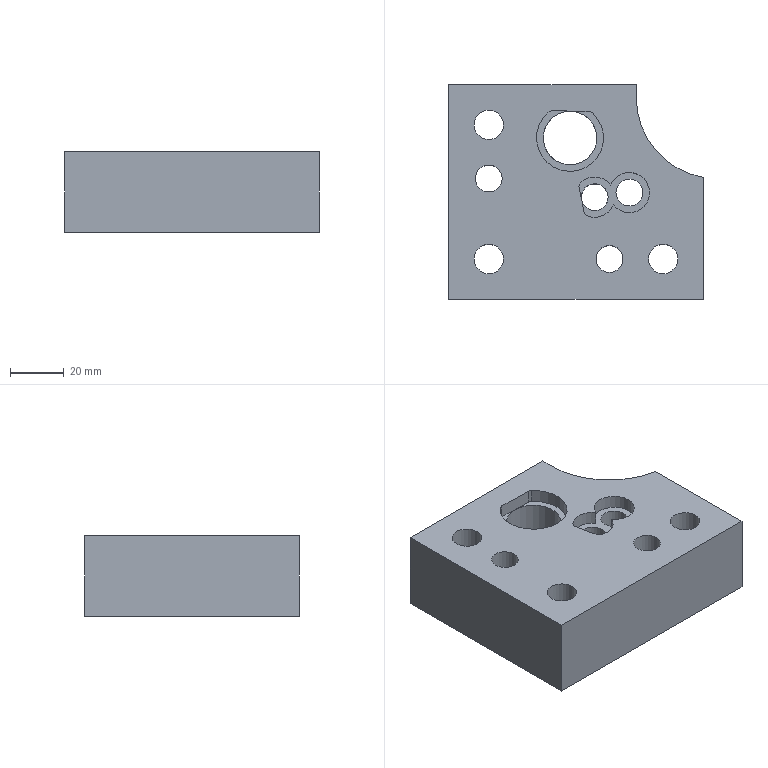Part | NX | features solid 2 | 1 solid | 34 faces | box 95 x 80 x 30 mm | volume 174573 mm3 | cylinder 20 | plane 14 | commonest cylinder face diameters 4 x4 10 x4 11 x3 15 x3 17 x3 20 x1
STEP:
#1=CARTESIAN_POINT('',(-403.57,200.221,109.));
#2=VERTEX_POINT('',#1);
#3=CARTESIAN_POINT('',(-404.546,207.571,109.));
#4=VERTEX_POINT('',#3);
#5=CARTESIAN_POINT('',(-397.595,204.754,109.));
#6=DIRECTION('',(0.,0.,-1.));
#7=DIRECTION('',(-1.,0.,0.));
#8=AXIS2_PLACEMENT_3D('',#5,#6,#7);
#9=CIRCLE('',#8,7.5);
#10=EDGE_CURVE('',#2,#4,#9,.F.);
#11=ORIENTED_EDGE('',*,*,#10,.F.);
#12=CARTESIAN_POINT('',(-413.225,196.042,109.));
#13=VERTEX_POINT('',#12);
#14=CARTESIAN_POINT('',(-410.521,203.038,109.));
#15=DIRECTION('',(0.,0.,-1.));
#16=DIRECTION('',(-1.,0.,0.));
#17=AXIS2_PLACEMENT_3D('',#14,#15,#16);
#18=CIRCLE('',#17,7.5);
#19=EDGE_CURVE('',#13,#2,#18,.F.);
#20=ORIENTED_EDGE('',*,*,#19,.F.);
#21=CARTESIAN_POINT('',(-414.461,197.494,109.));
#22=VERTEX_POINT('',#21);
#23=CARTESIAN_POINT('',(-412.504,197.908,109.));
#24=DIRECTION('',(0.,0.,-1.));
#25=DIRECTION('',(-1.,0.,0.));
#26=AXIS2_PLACEMENT_3D('',#23,#24,#25);
#27=CIRCLE('',#26,2.);
#28=EDGE_CURVE('',#13,#22,#27,.T.);
#29=ORIENTED_EDGE('',*,*,#28,.T.);
#30=CARTESIAN_POINT('',(-416.366,206.515,109.));
#31=VERTEX_POINT('',#30);
#32=CARTESIAN_POINT('',(-422.167,233.981,109.));
#33=DIRECTION('',(-0.2067,0.9784,0.));
#34=VECTOR('',#33,1000.);
#35=LINE('',#32,#34);
#36=EDGE_CURVE('',#22,#31,#35,.T.);
#37=ORIENTED_EDGE('',*,*,#36,.T.);
#38=CARTESIAN_POINT('',(-415.823,208.343,109.));
#39=VERTEX_POINT('',#38);
#40=CARTESIAN_POINT('',(-414.409,206.928,109.));
#41=DIRECTION('',(0.,0.,-1.));
#42=DIRECTION('',(-1.,0.,0.));
#43=AXIS2_PLACEMENT_3D('',#40,#41,#42);
#44=CIRCLE('',#43,2.);
#45=EDGE_CURVE('',#31,#39,#44,.T.);
#46=ORIENTED_EDGE('',*,*,#45,.T.);
#47=CARTESIAN_POINT('',(-410.521,203.038,109.));
#48=DIRECTION('',(0.,0.,-1.));
#49=DIRECTION('',(-1.,0.,0.));
#50=AXIS2_PLACEMENT_3D('',#47,#48,#49);
#51=CIRCLE('',#50,7.5);
#52=EDGE_CURVE('',#4,#39,#51,.F.);
#53=ORIENTED_EDGE('',*,*,#52,.F.);
#54=EDGE_LOOP('',(#11,#20,#29,#37,#46,#53));
#55=FACE_BOUND('',#54,.T.);
#56=CARTESIAN_POINT('',(-427.542,234.881,109.));
#57=VERTEX_POINT('',#56);
#58=CARTESIAN_POINT('',(-411.356,234.431,109.));
#59=VERTEX_POINT('',#58);
#60=CARTESIAN_POINT('',(-419.714,225.136,109.));
#61=DIRECTION('',(0.,0.,-1.));
#62=DIRECTION('',(-1.,0.,0.));
#63=AXIS2_PLACEMENT_3D('',#60,#61,#62);
#64=CIRCLE('',#63,12.5);
#65=EDGE_CURVE('',#57,#59,#64,.F.);
#66=ORIENTED_EDGE('',*,*,#65,.F.);
#67=CARTESIAN_POINT('',(-426.234,235.321,109.));
#68=VERTEX_POINT('',#67);
#69=CARTESIAN_POINT('',(-426.29,233.322,109.));
#70=DIRECTION('',(0.,0.,-1.));
#71=DIRECTION('',(-1.,0.,0.));
#72=AXIS2_PLACEMENT_3D('',#69,#70,#71);
#73=CIRCLE('',#72,2.);
#74=EDGE_CURVE('',#57,#68,#73,.T.);
#75=ORIENTED_EDGE('',*,*,#74,.T.);
#76=CARTESIAN_POINT('',(-412.638,234.943,109.));
#77=VERTEX_POINT('',#76);
#78=CARTESIAN_POINT('',(-370.312,233.766,109.));
#79=DIRECTION('',(0.9996,-0.0278,0.));
#80=VECTOR('',#79,1000.);
#81=LINE('',#78,#80);
#82=EDGE_CURVE('',#68,#77,#81,.T.);
#83=ORIENTED_EDGE('',*,*,#82,.T.);
#84=CARTESIAN_POINT('',(-412.693,232.944,109.));
#85=DIRECTION('',(0.,0.,-1.));
#86=DIRECTION('',(-1.,0.,0.));
#87=AXIS2_PLACEMENT_3D('',#84,#85,#86);
#88=CIRCLE('',#87,2.);
#89=EDGE_CURVE('',#77,#59,#88,.T.);
#90=ORIENTED_EDGE('',*,*,#89,.T.);
#91=EDGE_LOOP('',(#66,#75,#83,#90));
#92=FACE_BOUND('',#91,.T.);
#93=CARTESIAN_POINT('',(-455.5,180.,109.));
#94=VERTEX_POINT('',#93);
#95=CARTESIAN_POINT('',(-450.,180.,109.));
#96=DIRECTION('',(0.,0.,-1.));
#97=DIRECTION('',(-1.,0.,0.));
#98=AXIS2_PLACEMENT_3D('',#95,#96,#97);
#99=CIRCLE('',#98,5.5);
#100=EDGE_CURVE('',#94,#94,#99,.T.);
#101=ORIENTED_EDGE('',*,*,#100,.T.);
#102=EDGE_LOOP('',(#101));
#103=FACE_BOUND('',#102,.T.);
#104=CARTESIAN_POINT('',(-455.5,230.,109.));
#105=VERTEX_POINT('',#104);
#106=CARTESIAN_POINT('',(-450.,230.,109.));
#107=DIRECTION('',(0.,0.,-1.));
#108=DIRECTION('',(-1.,0.,0.));
#109=AXIS2_PLACEMENT_3D('',#106,#107,#108);
#110=CIRCLE('',#109,5.5);
#111=EDGE_CURVE('',#105,#105,#110,.T.);
#112=ORIENTED_EDGE('',*,*,#111,.T.);
#113=EDGE_LOOP('',(#112));
#114=FACE_BOUND('',#113,.T.);
#115=CARTESIAN_POINT('',(-390.5,180.,109.));
#116=VERTEX_POINT('',#115);
#117=CARTESIAN_POINT('',(-385.,180.,109.));
#118=DIRECTION('',(0.,0.,-1.));
#119=DIRECTION('',(-1.,0.,0.));
#120=AXIS2_PLACEMENT_3D('',#117,#118,#119);
#121=CIRCLE('',#120,5.5);
#122=EDGE_CURVE('',#116,#116,#121,.T.);
#123=ORIENTED_EDGE('',*,*,#122,.T.);
#124=EDGE_LOOP('',(#123));
#125=FACE_BOUND('',#124,.T.);
#126=CARTESIAN_POINT('',(-455.,210.,109.));
#127=VERTEX_POINT('',#126);
#128=CARTESIAN_POINT('',(-450.,210.,109.));
#129=DIRECTION('',(0.,0.,-1.));
#130=DIRECTION('',(-1.,0.,0.));
#131=AXIS2_PLACEMENT_3D('',#128,#129,#130);
#132=CIRCLE('',#131,5.);
#133=EDGE_CURVE('',#127,#127,#132,.T.);
#134=ORIENTED_EDGE('',*,*,#133,.T.);
#135=EDGE_LOOP('',(#134));
#136=FACE_BOUND('',#135,.T.);
#137=CARTESIAN_POINT('',(-410.,180.,109.));
#138=VERTEX_POINT('',#137);
#139=CARTESIAN_POINT('',(-405.,180.,109.));
#140=DIRECTION('',(0.,0.,-1.));
#141=DIRECTION('',(-1.,0.,0.));
#142=AXIS2_PLACEMENT_3D('',#139,#140,#141);
#143=CIRCLE('',#142,5.);
#144=EDGE_CURVE('',#138,#138,#143,.T.);
#145=ORIENTED_EDGE('',*,*,#144,.T.);
#146=EDGE_LOOP('',(#145));
#147=FACE_BOUND('',#146,.T.);
#148=CARTESIAN_POINT('',(-395.,245.,109.));
#149=VERTEX_POINT('',#148);
#150=CARTESIAN_POINT('',(-395.,240.,109.));
#151=VERTEX_POINT('',#150);
#152=CARTESIAN_POINT('',(-395.,245.,109.));
#153=DIRECTION('',(0.,-1.,0.));
#154=VECTOR('',#153,1000.);
#155=LINE('',#152,#154);
#156=EDGE_CURVE('',#149,#151,#155,.T.);
#157=ORIENTED_EDGE('',*,*,#156,.F.);
#158=CARTESIAN_POINT('',(-465.,245.,109.));
#159=VERTEX_POINT('',#158);
#160=CARTESIAN_POINT('',(-465.,245.,109.));
#161=DIRECTION('',(1.,0.,0.));
#162=VECTOR('',#161,1000.);
#163=LINE('',#160,#162);
#164=EDGE_CURVE('',#159,#149,#163,.T.);
#165=ORIENTED_EDGE('',*,*,#164,.F.);
#166=CARTESIAN_POINT('',(-465.,165.,109.));
#167=VERTEX_POINT('',#166);
#168=CARTESIAN_POINT('',(-465.,165.,109.));
#169=DIRECTION('',(0.,1.,0.));
#170=VECTOR('',#169,1000.);
#171=LINE('',#168,#170);
#172=EDGE_CURVE('',#167,#159,#171,.T.);
#173=ORIENTED_EDGE('',*,*,#172,.F.);
#174=CARTESIAN_POINT('',(-370.,165.,109.));
#175=VERTEX_POINT('',#174);
#176=CARTESIAN_POINT('',(-465.,165.,109.));
#177=DIRECTION('',(1.,0.,0.));
#178=VECTOR('',#177,1000.);
#179=LINE('',#176,#178);
#180=EDGE_CURVE('',#167,#175,#179,.T.);
#181=ORIENTED_EDGE('',*,*,#180,.T.);
#182=CARTESIAN_POINT('',(-370.,210.42,109.));
#183=VERTEX_POINT('',#182);
#184=CARTESIAN_POINT('',(-370.,165.,109.));
#185=DIRECTION('',(0.,1.,0.));
#186=VECTOR('',#185,1000.);
#187=LINE('',#184,#186);
#188=EDGE_CURVE('',#175,#183,#187,.T.);
#189=ORIENTED_EDGE('',*,*,#188,.T.);
#190=CARTESIAN_POINT('',(-365.,240.,109.));
#191=DIRECTION('',(0.,0.,-1.));
#192=DIRECTION('',(-1.,0.,0.));
#193=AXIS2_PLACEMENT_3D('',#190,#191,#192);
#194=CIRCLE('',#193,30.);
#195=EDGE_CURVE('',#183,#151,#194,.T.);
#196=ORIENTED_EDGE('',*,*,#195,.T.);
#197=EDGE_LOOP('',(#157,#165,#173,#181,#189,#196));
#198=FACE_BOUND('',#197,.T.);
#199=CARTESIAN_POINT('',(-370.,245.,109.));
#200=DIRECTION('',(0.,0.,-1.));
#201=DIRECTION('',(-1.,0.,0.));
#202=AXIS2_PLACEMENT_3D('',#199,#200,#201);
#203=PLANE('',#202);
#204=ADVANCED_FACE('',(#55,#92,#103,#114,#125,#136,#147,#198),#203,.F.);
#205=ORIENTED_EDGE('',*,*,#164,.T.);
#206=CARTESIAN_POINT('',(-395.,245.,79.));
#207=VERTEX_POINT('',#206);
#208=CARTESIAN_POINT('',(-395.,245.,109.));
#209=DIRECTION('',(0.,0.,-1.));
#210=VECTOR('',#209,1000.);
#211=LINE('',#208,#210);
#212=EDGE_CURVE('',#149,#207,#211,.T.);
#213=ORIENTED_EDGE('',*,*,#212,.T.);
#214=CARTESIAN_POINT('',(-465.,245.,79.));
#215=VERTEX_POINT('',#214);
#216=CARTESIAN_POINT('',(-465.,245.,79.));
#217=DIRECTION('',(1.,0.,0.));
#218=VECTOR('',#217,1000.);
#219=LINE('',#216,#218);
#220=EDGE_CURVE('',#215,#207,#219,.T.);
#221=ORIENTED_EDGE('',*,*,#220,.F.);
#222=CARTESIAN_POINT('',(-465.,245.,109.));
#223=DIRECTION('',(0.,0.,-1.));
#224=VECTOR('',#223,1000.);
#225=LINE('',#222,#224);
#226=EDGE_CURVE('',#159,#215,#225,.T.);
#227=ORIENTED_EDGE('',*,*,#226,.F.);
#228=EDGE_LOOP('',(#205,#213,#221,#227));
#229=FACE_BOUND('',#228,.T.);
#230=CARTESIAN_POINT('',(-465.,245.,109.));
#231=DIRECTION('',(0.,1.,0.));
#232=DIRECTION('',(0.,0.,1.));
#233=AXIS2_PLACEMENT_3D('',#230,#231,#232);
#234=PLANE('',#233);
#235=ADVANCED_FACE('',(#229),#234,.T.);
#236=CARTESIAN_POINT('',(-429.714,225.136,79.));
#237=VERTEX_POINT('',#236);
#238=CARTESIAN_POINT('',(-419.714,225.136,79.));
#239=DIRECTION('',(0.,0.,-1.));
#240=DIRECTION('',(-1.,0.,0.));
#241=AXIS2_PLACEMENT_3D('',#238,#239,#240);
#242=CIRCLE('',#241,10.);
#243=EDGE_CURVE('',#237,#237,#242,.T.);
#244=ORIENTED_EDGE('',*,*,#243,.F.);
#245=EDGE_LOOP('',(#244));
#246=FACE_BOUND('',#245,.T.);
#247=CARTESIAN_POINT('',(-415.521,203.038,79.));
#248=VERTEX_POINT('',#247);
#249=CARTESIAN_POINT('',(-410.521,203.038,79.));
#250=DIRECTION('',(0.,0.,-1.));
#251=DIRECTION('',(-1.,0.,0.));
#252=AXIS2_PLACEMENT_3D('',#249,#250,#251);
#253=CIRCLE('',#252,5.);
#254=EDGE_CURVE('',#248,#248,#253,.T.);
#255=ORIENTED_EDGE('',*,*,#254,.F.);
#256=EDGE_LOOP('',(#255));
#257=FACE_BOUND('',#256,.T.);
#258=CARTESIAN_POINT('',(-402.595,204.754,79.));
#259=VERTEX_POINT('',#258);
#260=CARTESIAN_POINT('',(-397.595,204.754,79.));
#261=DIRECTION('',(0.,0.,-1.));
#262=DIRECTION('',(-1.,0.,0.));
#263=AXIS2_PLACEMENT_3D('',#260,#261,#262);
#264=CIRCLE('',#263,5.);
#265=EDGE_CURVE('',#259,#259,#264,.T.);
#266=ORIENTED_EDGE('',*,*,#265,.F.);
#267=EDGE_LOOP('',(#266));
#268=FACE_BOUND('',#267,.T.);
#269=CARTESIAN_POINT('',(-458.5,180.,79.));
#270=VERTEX_POINT('',#269);
#271=CARTESIAN_POINT('',(-450.,180.,79.));
#272=DIRECTION('',(0.,0.,-1.));
#273=DIRECTION('',(-1.,0.,0.));
#274=AXIS2_PLACEMENT_3D('',#271,#272,#273);
#275=CIRCLE('',#274,8.5);
#276=EDGE_CURVE('',#270,#270,#275,.T.);
#277=ORIENTED_EDGE('',*,*,#276,.F.);
#278=EDGE_LOOP('',(#277));
#279=FACE_BOUND('',#278,.T.);
#280=CARTESIAN_POINT('',(-458.5,230.,79.));
#281=VERTEX_POINT('',#280);
#282=CARTESIAN_POINT('',(-450.,230.,79.));
#283=DIRECTION('',(0.,0.,-1.));
#284=DIRECTION('',(-1.,0.,0.));
#285=AXIS2_PLACEMENT_3D('',#282,#283,#284);
#286=CIRCLE('',#285,8.5);
#287=EDGE_CURVE('',#281,#281,#286,.T.);
#288=ORIENTED_EDGE('',*,*,#287,.F.);
#289=EDGE_LOOP('',(#288));
#290=FACE_BOUND('',#289,.T.);
#291=CARTESIAN_POINT('',(-393.5,180.,79.));
#292=VERTEX_POINT('',#291);
#293=CARTESIAN_POINT('',(-385.,180.,79.));
#294=DIRECTION('',(0.,0.,-1.));
#295=DIRECTION('',(-1.,0.,0.));
#296=AXIS2_PLACEMENT_3D('',#293,#294,#295);
#297=CIRCLE('',#296,8.5);
#298=EDGE_CURVE('',#292,#292,#297,.T.);
#299=ORIENTED_EDGE('',*,*,#298,.F.);
#300=EDGE_LOOP('',(#299));
#301=FACE_BOUND('',#300,.T.);
#302=CARTESIAN_POINT('',(-455.,210.,79.));
#303=VERTEX_POINT('',#302);
#304=CARTESIAN_POINT('',(-450.,210.,79.));
#305=DIRECTION('',(0.,0.,-1.));
#306=DIRECTION('',(-1.,0.,0.));
#307=AXIS2_PLACEMENT_3D('',#304,#305,#306);
#308=CIRCLE('',#307,5.);
#309=EDGE_CURVE('',#303,#303,#308,.T.);
#310=ORIENTED_EDGE('',*,*,#309,.F.);
#311=EDGE_LOOP('',(#310));
#312=FACE_BOUND('',#311,.T.);
#313=CARTESIAN_POINT('',(-410.,180.,79.));
#314=VERTEX_POINT('',#313);
#315=CARTESIAN_POINT('',(-405.,180.,79.));
#316=DIRECTION('',(0.,0.,-1.));
#317=DIRECTION('',(-1.,0.,0.));
#318=AXIS2_PLACEMENT_3D('',#315,#316,#317);
#319=CIRCLE('',#318,5.);
#320=EDGE_CURVE('',#314,#314,#319,.T.);
#321=ORIENTED_EDGE('',*,*,#320,.F.);
#322=EDGE_LOOP('',(#321));
#323=FACE_BOUND('',#322,.T.);
#324=ORIENTED_EDGE('',*,*,#220,.T.);
#325=CARTESIAN_POINT('',(-395.,240.,79.));
#326=VERTEX_POINT('',#325);
#327=CARTESIAN_POINT('',(-395.,245.,79.));
#328=DIRECTION('',(0.,-1.,0.));
#329=VECTOR('',#328,1000.);
#330=LINE('',#327,#329);
#331=EDGE_CURVE('',#207,#326,#330,.T.);
#332=ORIENTED_EDGE('',*,*,#331,.T.);
#333=CARTESIAN_POINT('',(-370.,210.42,79.));
#334=VERTEX_POINT('',#333);
#335=CARTESIAN_POINT('',(-365.,240.,79.));
#336=DIRECTION('',(0.,0.,-1.));
#337=DIRECTION('',(-1.,0.,0.));
#338=AXIS2_PLACEMENT_3D('',#335,#336,#337);
#339=CIRCLE('',#338,30.);
#340=EDGE_CURVE('',#334,#326,#339,.T.);
#341=ORIENTED_EDGE('',*,*,#340,.F.);
#342=CARTESIAN_POINT('',(-370.,165.,79.));
#343=VERTEX_POINT('',#342);
#344=CARTESIAN_POINT('',(-370.,165.,79.));
#345=DIRECTION('',(0.,1.,0.));
#346=VECTOR('',#345,1000.);
#347=LINE('',#344,#346);
#348=EDGE_CURVE('',#343,#334,#347,.T.);
#349=ORIENTED_EDGE('',*,*,#348,.F.);
#350=CARTESIAN_POINT('',(-465.,165.,79.));
#351=VERTEX_POINT('',#350);
#352=CARTESIAN_POINT('',(-465.,165.,79.));
#353=DIRECTION('',(1.,0.,0.));
#354=VECTOR('',#353,1000.);
#355=LINE('',#352,#354);
#356=EDGE_CURVE('',#351,#343,#355,.T.);
#357=ORIENTED_EDGE('',*,*,#356,.F.);
#358=CARTESIAN_POINT('',(-465.,165.,79.));
#359=DIRECTION('',(0.,1.,0.));
#360=VECTOR('',#359,1000.);
#361=LINE('',#358,#360);
#362=EDGE_CURVE('',#351,#215,#361,.T.);
#363=ORIENTED_EDGE('',*,*,#362,.T.);
#364=EDGE_LOOP('',(#324,#332,#341,#349,#357,#363));
#365=FACE_BOUND('',#364,.T.);
#366=CARTESIAN_POINT('',(-370.,245.,79.));
#367=DIRECTION('',(0.,0.,-1.));
#368=DIRECTION('',(-1.,0.,0.));
#369=AXIS2_PLACEMENT_3D('',#366,#367,#368);
#370=PLANE('',#369);
#371=ADVANCED_FACE('',(#246,#257,#268,#279,#290,#301,#312,#323,#365),#370,.T.);
#372=ORIENTED_EDGE('',*,*,#265,.T.);
#373=EDGE_LOOP('',(#372));
#374=FACE_BOUND('',#373,.T.);
#375=CARTESIAN_POINT('',(-392.595,204.754,104.));
#376=VERTEX_POINT('',#375);
#377=CARTESIAN_POINT('',(-397.595,204.754,104.));
#378=DIRECTION('',(0.,0.,1.));
#379=DIRECTION('',(1.,0.,0.));
#380=AXIS2_PLACEMENT_3D('',#377,#378,#379);
#381=CIRCLE('',#380,5.);
#382=EDGE_CURVE('',#376,#376,#381,.F.);
#383=ORIENTED_EDGE('',*,*,#382,.F.);
#384=EDGE_LOOP('',(#383));
#385=FACE_BOUND('',#384,.T.);
#386=CARTESIAN_POINT('',(-397.595,204.754,-452.));
#387=DIRECTION('',(0.,0.,1.));
#388=DIRECTION('',(1.,0.,0.));
#389=AXIS2_PLACEMENT_3D('',#386,#387,#388);
#390=CYLINDRICAL_SURFACE('',#389,5.);
#391=ADVANCED_FACE('',(#374,#385),#390,.F.);
#392=CARTESIAN_POINT('',(-413.225,196.042,104.));
#393=VERTEX_POINT('',#392);
#394=CARTESIAN_POINT('',(-403.57,200.221,104.));
#395=VERTEX_POINT('',#394);
#396=CARTESIAN_POINT('',(-410.521,203.038,104.));
#397=DIRECTION('',(0.,0.,1.));
#398=DIRECTION('',(1.,0.,0.));
#399=AXIS2_PLACEMENT_3D('',#396,#397,#398);
#400=CIRCLE('',#399,7.5);
#401=EDGE_CURVE('',#393,#395,#400,.T.);
#402=ORIENTED_EDGE('',*,*,#401,.F.);
#403=CARTESIAN_POINT('',(-413.225,196.042,104.));
#404=DIRECTION('',(0.,0.,-1.));
#405=VECTOR('',#404,1000.);
#406=LINE('',#403,#405);
#407=EDGE_CURVE('',#393,#13,#406,.F.);
#408=ORIENTED_EDGE('',*,*,#407,.T.);
#409=ORIENTED_EDGE('',*,*,#19,.T.);
#410=CARTESIAN_POINT('',(-403.57,200.221,206.5));
#411=DIRECTION('',(0.,0.,-1.));
#412=VECTOR('',#411,1000.);
#413=LINE('',#410,#412);
#414=EDGE_CURVE('',#2,#395,#413,.T.);
#415=ORIENTED_EDGE('',*,*,#414,.T.);
#416=EDGE_LOOP('',(#402,#408,#409,#415));
#417=FACE_BOUND('',#416,.T.);
#418=CARTESIAN_POINT('',(-410.521,203.038,309.));
#419=DIRECTION('',(0.,0.,-1.));
#420=DIRECTION('',(-1.,0.,0.));
#421=AXIS2_PLACEMENT_3D('',#418,#419,#420);
#422=CYLINDRICAL_SURFACE('',#421,7.5);
#423=ADVANCED_FACE('',(#417),#422,.F.);
#424=ORIENTED_EDGE('',*,*,#52,.T.);
#425=CARTESIAN_POINT('',(-415.823,208.343,104.));
#426=VERTEX_POINT('',#425);
#427=CARTESIAN_POINT('',(-415.823,208.343,109.));
#428=DIRECTION('',(0.,0.,-1.));
#429=VECTOR('',#428,1000.);
#430=LINE('',#427,#429);
#431=EDGE_CURVE('',#39,#426,#430,.T.);
#432=ORIENTED_EDGE('',*,*,#431,.T.);
#433=CARTESIAN_POINT('',(-404.546,207.571,104.));
#434=VERTEX_POINT('',#433);
#435=CARTESIAN_POINT('',(-410.521,203.038,104.));
#436=DIRECTION('',(0.,0.,1.));
#437=DIRECTION('',(1.,0.,0.));
#438=AXIS2_PLACEMENT_3D('',#435,#436,#437);
#439=CIRCLE('',#438,7.5);
#440=EDGE_CURVE('',#434,#426,#439,.T.);
#441=ORIENTED_EDGE('',*,*,#440,.F.);
#442=CARTESIAN_POINT('',(-404.546,207.571,206.5));
#443=DIRECTION('',(0.,0.,-1.));
#444=VECTOR('',#443,1000.);
#445=LINE('',#442,#444);
#446=EDGE_CURVE('',#434,#4,#445,.F.);
#447=ORIENTED_EDGE('',*,*,#446,.T.);
#448=EDGE_LOOP('',(#424,#432,#441,#447));
#449=FACE_BOUND('',#448,.T.);
#450=CARTESIAN_POINT('',(-410.521,203.038,309.));
#451=DIRECTION('',(0.,0.,-1.));
#452=DIRECTION('',(-1.,0.,0.));
#453=AXIS2_PLACEMENT_3D('',#450,#451,#452);
#454=CYLINDRICAL_SURFACE('',#453,7.5);
#455=ADVANCED_FACE('',(#449),#454,.F.);
#456=ORIENTED_EDGE('',*,*,#254,.T.);
#457=EDGE_LOOP('',(#456));
#458=FACE_BOUND('',#457,.T.);
#459=CARTESIAN_POINT('',(-415.413,202.004,104.));
#460=VERTEX_POINT('',#459);
#461=CARTESIAN_POINT('',(-410.521,203.038,104.));
#462=DIRECTION('',(0.,0.,1.));
#463=DIRECTION('',(1.,0.,0.));
#464=AXIS2_PLACEMENT_3D('',#461,#462,#463);
#465=CIRCLE('',#464,5.);
#466=EDGE_CURVE('',#460,#460,#465,.F.);
#467=ORIENTED_EDGE('',*,*,#466,.F.);
#468=EDGE_LOOP('',(#467));
#469=FACE_BOUND('',#468,.T.);
#470=CARTESIAN_POINT('',(-410.521,203.038,-452.));
#471=DIRECTION('',(0.,0.,1.));
#472=DIRECTION('',(1.,0.,0.));
#473=AXIS2_PLACEMENT_3D('',#470,#471,#472);
#474=CYLINDRICAL_SURFACE('',#473,5.);
#475=ADVANCED_FACE('',(#458,#469),#474,.F.);
#476=ORIENTED_EDGE('',*,*,#243,.T.);
#477=EDGE_LOOP('',(#476));
#478=FACE_BOUND('',#477,.T.);
#479=CARTESIAN_POINT('',(-419.436,235.132,104.));
#480=VERTEX_POINT('',#479);
#481=CARTESIAN_POINT('',(-419.714,225.136,104.));
#482=DIRECTION('',(0.,0.,1.));
#483=DIRECTION('',(1.,0.,0.));
#484=AXIS2_PLACEMENT_3D('',#481,#482,#483);
#485=CIRCLE('',#484,10.);
#486=EDGE_CURVE('',#480,#480,#485,.F.);
#487=ORIENTED_EDGE('',*,*,#486,.F.);
#488=EDGE_LOOP('',(#487));
#489=FACE_BOUND('',#488,.T.);
#490=CARTESIAN_POINT('',(-419.714,225.136,-446.));
#491=DIRECTION('',(0.,0.,1.));
#492=DIRECTION('',(1.,0.,0.));
#493=AXIS2_PLACEMENT_3D('',#490,#491,#492);
#494=CYLINDRICAL_SURFACE('',#493,10.);
#495=ADVANCED_FACE('',(#478,#489),#494,.F.);
#496=ORIENTED_EDGE('',*,*,#348,.T.);
#497=CARTESIAN_POINT('',(-370.,210.42,-421.));
#498=DIRECTION('',(0.,0.,1.));
#499=VECTOR('',#498,1000.);
#500=LINE('',#497,#499);
#501=EDGE_CURVE('',#334,#183,#500,.T.);
#502=ORIENTED_EDGE('',*,*,#501,.T.);
#503=ORIENTED_EDGE('',*,*,#188,.F.);
#504=CARTESIAN_POINT('',(-370.,165.,109.));
#505=DIRECTION('',(0.,0.,-1.));
#506=VECTOR('',#505,1000.);
#507=LINE('',#504,#506);
#508=EDGE_CURVE('',#175,#343,#507,.T.);
#509=ORIENTED_EDGE('',*,*,#508,.T.);
#510=EDGE_LOOP('',(#496,#502,#503,#509));
#511=FACE_BOUND('',#510,.T.);
#512=CARTESIAN_POINT('',(-370.,165.,109.));
#513=DIRECTION('',(-1.,0.,0.));
#514=DIRECTION('',(0.,0.,1.));
#515=AXIS2_PLACEMENT_3D('',#512,#513,#514);
#516=PLANE('',#515);
#517=ADVANCED_FACE('',(#511),#516,.F.);
#518=ORIENTED_EDGE('',*,*,#362,.F.);
#519=CARTESIAN_POINT('',(-465.,165.,109.));
#520=DIRECTION('',(0.,0.,-1.));
#521=VECTOR('',#520,1000.);
#522=LINE('',#519,#521);
#523=EDGE_CURVE('',#167,#351,#522,.T.);
#524=ORIENTED_EDGE('',*,*,#523,.F.);
#525=ORIENTED_EDGE('',*,*,#172,.T.);
#526=ORIENTED_EDGE('',*,*,#226,.T.);
#527=EDGE_LOOP('',(#518,#524,#525,#526));
#528=FACE_BOUND('',#527,.T.);
#529=CARTESIAN_POINT('',(-465.,165.,109.));
#530=DIRECTION('',(-1.,0.,0.));
#531=DIRECTION('',(0.,0.,1.));
#532=AXIS2_PLACEMENT_3D('',#529,#530,#531);
#533=PLANE('',#532);
#534=ADVANCED_FACE('',(#528),#533,.T.);
#535=ORIENTED_EDGE('',*,*,#356,.T.);
#536=ORIENTED_EDGE('',*,*,#508,.F.);
#537=ORIENTED_EDGE('',*,*,#180,.F.);
#538=ORIENTED_EDGE('',*,*,#523,.T.);
#539=EDGE_LOOP('',(#535,#536,#537,#538));
#540=FACE_BOUND('',#539,.T.);
#541=CARTESIAN_POINT('',(-465.,165.,109.));
#542=DIRECTION('',(0.,1.,0.));
#543=DIRECTION('',(0.,0.,1.));
#544=AXIS2_PLACEMENT_3D('',#541,#542,#543);
#545=PLANE('',#544);
#546=ADVANCED_FACE('',(#540),#545,.F.);
#547=ORIENTED_EDGE('',*,*,#65,.T.);
#548=CARTESIAN_POINT('',(-411.356,234.431,104.));
#549=VERTEX_POINT('',#548);
#550=CARTESIAN_POINT('',(-411.356,234.431,109.));
#551=DIRECTION('',(0.,0.,-1.));
#552=VECTOR('',#551,1000.);
#553=LINE('',#550,#552);
#554=EDGE_CURVE('',#59,#549,#553,.T.);
#555=ORIENTED_EDGE('',*,*,#554,.T.);
#556=CARTESIAN_POINT('',(-427.542,234.881,104.));
#557=VERTEX_POINT('',#556);
#558=CARTESIAN_POINT('',(-419.714,225.136,104.));
#559=DIRECTION('',(0.,0.,1.));
#560=DIRECTION('',(1.,0.,0.));
#561=AXIS2_PLACEMENT_3D('',#558,#559,#560);
#562=CIRCLE('',#561,12.5);
#563=EDGE_CURVE('',#557,#549,#562,.T.);
#564=ORIENTED_EDGE('',*,*,#563,.F.);
#565=CARTESIAN_POINT('',(-427.542,234.881,104.));
#566=DIRECTION('',(0.,0.,-1.));
#567=VECTOR('',#566,1000.);
#568=LINE('',#565,#567);
#569=EDGE_CURVE('',#557,#57,#568,.F.);
#570=ORIENTED_EDGE('',*,*,#569,.T.);
#571=EDGE_LOOP('',(#547,#555,#564,#570));
#572=FACE_BOUND('',#571,.T.);
#573=CARTESIAN_POINT('',(-419.714,225.136,309.));
#574=DIRECTION('',(0.,0.,-1.));
#575=DIRECTION('',(-1.,0.,0.));
#576=AXIS2_PLACEMENT_3D('',#573,#574,#575);
#577=CYLINDRICAL_SURFACE('',#576,12.5);
#578=ADVANCED_FACE('',(#572),#577,.F.);
#579=CARTESIAN_POINT('',(-412.638,234.943,104.));
#580=VERTEX_POINT('',#579);
#581=CARTESIAN_POINT('',(-419.436,235.132,104.));
#582=DIRECTION('',(0.9996,-0.0278,0.));
#583=VECTOR('',#582,1000.);
#584=LINE('',#581,#583);
#585=EDGE_CURVE('',#480,#580,#584,.T.);
#586=ORIENTED_EDGE('',*,*,#585,.T.);
#587=CARTESIAN_POINT('',(-412.638,234.943,309.));
#588=DIRECTION('',(0.,0.,-1.));
#589=VECTOR('',#588,1000.);
#590=LINE('',#587,#589);
#591=EDGE_CURVE('',#580,#77,#590,.F.);
#592=ORIENTED_EDGE('',*,*,#591,.T.);
#593=ORIENTED_EDGE('',*,*,#82,.F.);
#594=CARTESIAN_POINT('',(-426.234,235.321,104.));
#595=VERTEX_POINT('',#594);
#596=CARTESIAN_POINT('',(-426.234,235.321,309.));
#597=DIRECTION('',(0.,0.,-1.));
#598=VECTOR('',#597,1000.);
#599=LINE('',#596,#598);
#600=EDGE_CURVE('',#68,#595,#599,.T.);
#601=ORIENTED_EDGE('',*,*,#600,.T.);
#602=CARTESIAN_POINT('',(-419.436,235.132,104.));
#603=DIRECTION('',(0.9996,-0.0278,0.));
#604=VECTOR('',#603,1000.);
#605=LINE('',#602,#604);
#606=EDGE_CURVE('',#595,#480,#605,.T.);
#607=ORIENTED_EDGE('',*,*,#606,.T.);
#608=EDGE_LOOP('',(#586,#592,#593,#601,#607));
#609=FACE_BOUND('',#608,.T.);
#610=CARTESIAN_POINT('',(-419.436,235.132,309.));
#611=DIRECTION('',(0.0278,0.9996,0.));
#612=DIRECTION('',(-0.9996,0.0278,0.));
#613=AXIS2_PLACEMENT_3D('',#610,#611,#612);
#614=PLANE('',#613);
#615=ADVANCED_FACE('',(#609),#614,.F.);
#616=ORIENTED_EDGE('',*,*,#563,.T.);
#617=CARTESIAN_POINT('',(-412.693,232.944,104.));
#618=DIRECTION('',(0.,0.,1.));
#619=DIRECTION('',(1.,0.,0.));
#620=AXIS2_PLACEMENT_3D('',#617,#618,#619);
#621=CIRCLE('',#620,2.);
#622=EDGE_CURVE('',#549,#580,#621,.T.);
#623=ORIENTED_EDGE('',*,*,#622,.T.);
#624=ORIENTED_EDGE('',*,*,#585,.F.);
#625=ORIENTED_EDGE('',*,*,#486,.T.);
#626=ORIENTED_EDGE('',*,*,#606,.F.);
#627=CARTESIAN_POINT('',(-426.29,233.322,104.));
#628=DIRECTION('',(0.,0.,1.));
#629=DIRECTION('',(1.,0.,0.));
#630=AXIS2_PLACEMENT_3D('',#627,#628,#629);
#631=CIRCLE('',#630,2.);
#632=EDGE_CURVE('',#595,#557,#631,.T.);
#633=ORIENTED_EDGE('',*,*,#632,.T.);
#634=EDGE_LOOP('',(#616,#623,#624,#625,#626,#633));
#635=FACE_BOUND('',#634,.T.);
#636=CARTESIAN_POINT('',(-419.714,225.136,104.));
#637=DIRECTION('',(0.,0.,1.));
#638=DIRECTION('',(-0.0278,-0.9996,0.));
#639=AXIS2_PLACEMENT_3D('',#636,#637,#638);
#640=PLANE('',#639);
#641=ADVANCED_FACE('',(#635),#640,.T.);
#642=CARTESIAN_POINT('',(-416.366,206.515,104.));
#643=VERTEX_POINT('',#642);
#644=CARTESIAN_POINT('',(-415.413,202.004,104.));
#645=DIRECTION('',(-0.2067,0.9784,0.));
#646=VECTOR('',#645,1000.);
#647=LINE('',#644,#646);
#648=EDGE_CURVE('',#460,#643,#647,.T.);
#649=ORIENTED_EDGE('',*,*,#648,.T.);
#650=CARTESIAN_POINT('',(-416.366,206.515,309.));
#651=DIRECTION('',(0.,0.,-1.));
#652=VECTOR('',#651,1000.);
#653=LINE('',#650,#652);
#654=EDGE_CURVE('',#643,#31,#653,.F.);
#655=ORIENTED_EDGE('',*,*,#654,.T.);
#656=ORIENTED_EDGE('',*,*,#36,.F.);
#657=CARTESIAN_POINT('',(-414.461,197.494,104.));
#658=VERTEX_POINT('',#657);
#659=CARTESIAN_POINT('',(-414.461,197.494,309.));
#660=DIRECTION('',(0.,0.,-1.));
#661=VECTOR('',#660,1000.);
#662=LINE('',#659,#661);
#663=EDGE_CURVE('',#22,#658,#662,.T.);
#664=ORIENTED_EDGE('',*,*,#663,.T.);
#665=CARTESIAN_POINT('',(-415.413,202.004,104.));
#666=DIRECTION('',(-0.2067,0.9784,0.));
#667=VECTOR('',#666,1000.);
#668=LINE('',#665,#667);
#669=EDGE_CURVE('',#658,#460,#668,.T.);
#670=ORIENTED_EDGE('',*,*,#669,.T.);
#671=EDGE_LOOP('',(#649,#655,#656,#664,#670));
#672=FACE_BOUND('',#671,.T.);
#673=CARTESIAN_POINT('',(-415.413,202.004,309.));
#674=DIRECTION('',(-0.9784,-0.2067,0.));
#675=DIRECTION('',(0.2067,-0.9784,0.));
#676=AXIS2_PLACEMENT_3D('',#673,#674,#675);
#677=PLANE('',#676);
#678=ADVANCED_FACE('',(#672),#677,.F.);
#679=ORIENTED_EDGE('',*,*,#440,.T.);
#680=CARTESIAN_POINT('',(-414.409,206.928,104.));
#681=DIRECTION('',(0.,0.,1.));
#682=DIRECTION('',(1.,0.,0.));
#683=AXIS2_PLACEMENT_3D('',#680,#681,#682);
#684=CIRCLE('',#683,2.);
#685=EDGE_CURVE('',#426,#643,#684,.T.);
#686=ORIENTED_EDGE('',*,*,#685,.T.);
#687=ORIENTED_EDGE('',*,*,#648,.F.);
#688=ORIENTED_EDGE('',*,*,#466,.T.);
#689=ORIENTED_EDGE('',*,*,#669,.F.);
#690=CARTESIAN_POINT('',(-412.504,197.908,104.));
#691=DIRECTION('',(0.,0.,1.));
#692=DIRECTION('',(1.,0.,0.));
#693=AXIS2_PLACEMENT_3D('',#690,#691,#692);
#694=CIRCLE('',#693,2.);
#695=EDGE_CURVE('',#658,#393,#694,.T.);
#696=ORIENTED_EDGE('',*,*,#695,.T.);
#697=ORIENTED_EDGE('',*,*,#401,.T.);
#698=CARTESIAN_POINT('',(-397.595,204.754,104.));
#699=DIRECTION('',(0.,0.,1.));
#700=DIRECTION('',(1.,0.,0.));
#701=AXIS2_PLACEMENT_3D('',#698,#699,#700);
#702=CIRCLE('',#701,7.5);
#703=EDGE_CURVE('',#395,#434,#702,.T.);
#704=ORIENTED_EDGE('',*,*,#703,.T.);
#705=EDGE_LOOP('',(#679,#686,#687,#688,#689,#696,#697,#704));
#706=FACE_BOUND('',#705,.T.);
#707=ORIENTED_EDGE('',*,*,#382,.T.);
#708=EDGE_LOOP('',(#707));
#709=FACE_BOUND('',#708,.T.);
#710=CARTESIAN_POINT('',(-410.521,203.038,104.));
#711=DIRECTION('',(0.,0.,1.));
#712=DIRECTION('',(0.9784,0.2067,0.));
#713=AXIS2_PLACEMENT_3D('',#710,#711,#712);
#714=PLANE('',#713);
#715=ADVANCED_FACE('',(#706,#709),#714,.T.);
#716=ORIENTED_EDGE('',*,*,#10,.T.);
#717=ORIENTED_EDGE('',*,*,#446,.F.);
#718=ORIENTED_EDGE('',*,*,#703,.F.);
#719=ORIENTED_EDGE('',*,*,#414,.F.);
#720=EDGE_LOOP('',(#716,#717,#718,#719));
#721=FACE_BOUND('',#720,.T.);
#722=CARTESIAN_POINT('',(-397.595,204.754,309.));
#723=DIRECTION('',(0.,0.,-1.));
#724=DIRECTION('',(-1.,0.,0.));
#725=AXIS2_PLACEMENT_3D('',#722,#723,#724);
#726=CYLINDRICAL_SURFACE('',#725,7.5);
#727=ADVANCED_FACE('',(#721),#726,.F.);
#728=ORIENTED_EDGE('',*,*,#74,.F.);
#729=ORIENTED_EDGE('',*,*,#569,.F.);
#730=ORIENTED_EDGE('',*,*,#632,.F.);
#731=ORIENTED_EDGE('',*,*,#600,.F.);
#732=EDGE_LOOP('',(#728,#729,#730,#731));
#733=FACE_BOUND('',#732,.T.);
#734=CARTESIAN_POINT('',(-426.29,233.322,309.));
#735=DIRECTION('',(0.,0.,-1.));
#736=DIRECTION('',(-1.,0.,0.));
#737=AXIS2_PLACEMENT_3D('',#734,#735,#736);
#738=CYLINDRICAL_SURFACE('',#737,2.);
#739=ADVANCED_FACE('',(#733),#738,.F.);
#740=ORIENTED_EDGE('',*,*,#89,.F.);
#741=ORIENTED_EDGE('',*,*,#591,.F.);
#742=ORIENTED_EDGE('',*,*,#622,.F.);
#743=ORIENTED_EDGE('',*,*,#554,.F.);
#744=EDGE_LOOP('',(#740,#741,#742,#743));
#745=FACE_BOUND('',#744,.T.);
#746=CARTESIAN_POINT('',(-412.693,232.944,309.));
#747=DIRECTION('',(0.,0.,-1.));
#748=DIRECTION('',(-1.,0.,0.));
#749=AXIS2_PLACEMENT_3D('',#746,#747,#748);
#750=CYLINDRICAL_SURFACE('',#749,2.);
#751=ADVANCED_FACE('',(#745),#750,.F.);
#752=ORIENTED_EDGE('',*,*,#28,.F.);
#753=ORIENTED_EDGE('',*,*,#407,.F.);
#754=ORIENTED_EDGE('',*,*,#695,.F.);
#755=ORIENTED_EDGE('',*,*,#663,.F.);
#756=EDGE_LOOP('',(#752,#753,#754,#755));
#757=FACE_BOUND('',#756,.T.);
#758=CARTESIAN_POINT('',(-412.504,197.908,309.));
#759=DIRECTION('',(0.,0.,-1.));
#760=DIRECTION('',(-1.,0.,0.));
#761=AXIS2_PLACEMENT_3D('',#758,#759,#760);
#762=CYLINDRICAL_SURFACE('',#761,2.);
#763=ADVANCED_FACE('',(#757),#762,.F.);
#764=ORIENTED_EDGE('',*,*,#45,.F.);
#765=ORIENTED_EDGE('',*,*,#654,.F.);
#766=ORIENTED_EDGE('',*,*,#685,.F.);
#767=ORIENTED_EDGE('',*,*,#431,.F.);
#768=EDGE_LOOP('',(#764,#765,#766,#767));
#769=FACE_BOUND('',#768,.T.);
#770=CARTESIAN_POINT('',(-414.409,206.928,309.));
#771=DIRECTION('',(0.,0.,-1.));
#772=DIRECTION('',(-1.,0.,0.));
#773=AXIS2_PLACEMENT_3D('',#770,#771,#772);
#774=CYLINDRICAL_SURFACE('',#773,2.);
#775=ADVANCED_FACE('',(#769),#774,.F.);
#776=CARTESIAN_POINT('',(-444.5,180.,89.));
#777=VERTEX_POINT('',#776);
#778=CARTESIAN_POINT('',(-450.,180.,89.));
#779=DIRECTION('',(0.,0.,1.));
#780=DIRECTION('',(1.,0.,0.));
#781=AXIS2_PLACEMENT_3D('',#778,#779,#780);
#782=CIRCLE('',#781,5.5);
#783=EDGE_CURVE('',#777,#777,#782,.F.);
#784=ORIENTED_EDGE('',*,*,#783,.T.);
#785=EDGE_LOOP('',(#784));
#786=FACE_BOUND('',#785,.T.);
#787=ORIENTED_EDGE('',*,*,#100,.F.);
#788=EDGE_LOOP('',(#787));
#789=FACE_BOUND('',#788,.T.);
#790=CARTESIAN_POINT('',(-450.,180.,129.));
#791=DIRECTION('',(0.,0.,-1.));
#792=DIRECTION('',(-1.,0.,0.));
#793=AXIS2_PLACEMENT_3D('',#790,#791,#792);
#794=CYLINDRICAL_SURFACE('',#793,5.5);
#795=ADVANCED_FACE('',(#786,#789),#794,.F.);
#796=ORIENTED_EDGE('',*,*,#783,.F.);
#797=EDGE_LOOP('',(#796));
#798=FACE_BOUND('',#797,.T.);
#799=CARTESIAN_POINT('',(-458.5,180.,89.));
#800=VERTEX_POINT('',#799);
#801=CARTESIAN_POINT('',(-450.,180.,89.));
#802=DIRECTION('',(0.,0.,-1.));
#803=DIRECTION('',(-1.,0.,0.));
#804=AXIS2_PLACEMENT_3D('',#801,#802,#803);
#805=CIRCLE('',#804,8.5);
#806=EDGE_CURVE('',#800,#800,#805,.T.);
#807=ORIENTED_EDGE('',*,*,#806,.T.);
#808=EDGE_LOOP('',(#807));
#809=FACE_BOUND('',#808,.T.);
#810=CARTESIAN_POINT('',(-450.,180.,89.));
#811=DIRECTION('',(0.,0.,1.));
#812=DIRECTION('',(1.,0.,0.));
#813=AXIS2_PLACEMENT_3D('',#810,#811,#812);
#814=PLANE('',#813);
#815=ADVANCED_FACE('',(#798,#809),#814,.F.);
#816=ORIENTED_EDGE('',*,*,#276,.T.);
#817=EDGE_LOOP('',(#816));
#818=FACE_BOUND('',#817,.T.);
#819=ORIENTED_EDGE('',*,*,#806,.F.);
#820=EDGE_LOOP('',(#819));
#821=FACE_BOUND('',#820,.T.);
#822=CARTESIAN_POINT('',(-450.,180.,89.));
#823=DIRECTION('',(0.,0.,-1.));
#824=DIRECTION('',(-1.,0.,0.));
#825=AXIS2_PLACEMENT_3D('',#822,#823,#824);
#826=CYLINDRICAL_SURFACE('',#825,8.5);
#827=ADVANCED_FACE('',(#818,#821),#826,.F.);
#828=CARTESIAN_POINT('',(-444.5,230.,89.));
#829=VERTEX_POINT('',#828);
#830=CARTESIAN_POINT('',(-450.,230.,89.));
#831=DIRECTION('',(0.,0.,1.));
#832=DIRECTION('',(1.,0.,0.));
#833=AXIS2_PLACEMENT_3D('',#830,#831,#832);
#834=CIRCLE('',#833,5.5);
#835=EDGE_CURVE('',#829,#829,#834,.F.);
#836=ORIENTED_EDGE('',*,*,#835,.T.);
#837=EDGE_LOOP('',(#836));
#838=FACE_BOUND('',#837,.T.);
#839=ORIENTED_EDGE('',*,*,#111,.F.);
#840=EDGE_LOOP('',(#839));
#841=FACE_BOUND('',#840,.T.);
#842=CARTESIAN_POINT('',(-450.,230.,129.));
#843=DIRECTION('',(0.,0.,-1.));
#844=DIRECTION('',(-1.,0.,0.));
#845=AXIS2_PLACEMENT_3D('',#842,#843,#844);
#846=CYLINDRICAL_SURFACE('',#845,5.5);
#847=ADVANCED_FACE('',(#838,#841),#846,.F.);
#848=ORIENTED_EDGE('',*,*,#835,.F.);
#849=EDGE_LOOP('',(#848));
#850=FACE_BOUND('',#849,.T.);
#851=CARTESIAN_POINT('',(-458.5,230.,89.));
#852=VERTEX_POINT('',#851);
#853=CARTESIAN_POINT('',(-450.,230.,89.));
#854=DIRECTION('',(0.,0.,-1.));
#855=DIRECTION('',(-1.,0.,0.));
#856=AXIS2_PLACEMENT_3D('',#853,#854,#855);
#857=CIRCLE('',#856,8.5);
#858=EDGE_CURVE('',#852,#852,#857,.T.);
#859=ORIENTED_EDGE('',*,*,#858,.T.);
#860=EDGE_LOOP('',(#859));
#861=FACE_BOUND('',#860,.T.);
#862=CARTESIAN_POINT('',(-450.,230.,89.));
#863=DIRECTION('',(0.,0.,1.));
#864=DIRECTION('',(1.,0.,0.));
#865=AXIS2_PLACEMENT_3D('',#862,#863,#864);
#866=PLANE('',#865);
#867=ADVANCED_FACE('',(#850,#861),#866,.F.);
#868=ORIENTED_EDGE('',*,*,#287,.T.);
#869=EDGE_LOOP('',(#868));
#870=FACE_BOUND('',#869,.T.);
#871=ORIENTED_EDGE('',*,*,#858,.F.);
#872=EDGE_LOOP('',(#871));
#873=FACE_BOUND('',#872,.T.);
#874=CARTESIAN_POINT('',(-450.,230.,89.));
#875=DIRECTION('',(0.,0.,-1.));
#876=DIRECTION('',(-1.,0.,0.));
#877=AXIS2_PLACEMENT_3D('',#874,#875,#876);
#878=CYLINDRICAL_SURFACE('',#877,8.5);
#879=ADVANCED_FACE('',(#870,#873),#878,.F.);
#880=CARTESIAN_POINT('',(-379.5,180.,89.));
#881=VERTEX_POINT('',#880);
#882=CARTESIAN_POINT('',(-385.,180.,89.));
#883=DIRECTION('',(0.,0.,1.));
#884=DIRECTION('',(1.,0.,0.));
#885=AXIS2_PLACEMENT_3D('',#882,#883,#884);
#886=CIRCLE('',#885,5.5);
#887=EDGE_CURVE('',#881,#881,#886,.F.);
#888=ORIENTED_EDGE('',*,*,#887,.T.);
#889=EDGE_LOOP('',(#888));
#890=FACE_BOUND('',#889,.T.);
#891=ORIENTED_EDGE('',*,*,#122,.F.);
#892=EDGE_LOOP('',(#891));
#893=FACE_BOUND('',#892,.T.);
#894=CARTESIAN_POINT('',(-385.,180.,129.));
#895=DIRECTION('',(0.,0.,-1.));
#896=DIRECTION('',(-1.,0.,0.));
#897=AXIS2_PLACEMENT_3D('',#894,#895,#896);
#898=CYLINDRICAL_SURFACE('',#897,5.5);
#899=ADVANCED_FACE('',(#890,#893),#898,.F.);
#900=ORIENTED_EDGE('',*,*,#887,.F.);
#901=EDGE_LOOP('',(#900));
#902=FACE_BOUND('',#901,.T.);
#903=CARTESIAN_POINT('',(-393.5,180.,89.));
#904=VERTEX_POINT('',#903);
#905=CARTESIAN_POINT('',(-385.,180.,89.));
#906=DIRECTION('',(0.,0.,-1.));
#907=DIRECTION('',(-1.,0.,0.));
#908=AXIS2_PLACEMENT_3D('',#905,#906,#907);
#909=CIRCLE('',#908,8.5);
#910=EDGE_CURVE('',#904,#904,#909,.T.);
#911=ORIENTED_EDGE('',*,*,#910,.T.);
#912=EDGE_LOOP('',(#911));
#913=FACE_BOUND('',#912,.T.);
#914=CARTESIAN_POINT('',(-385.,180.,89.));
#915=DIRECTION('',(0.,0.,1.));
#916=DIRECTION('',(1.,0.,0.));
#917=AXIS2_PLACEMENT_3D('',#914,#915,#916);
#918=PLANE('',#917);
#919=ADVANCED_FACE('',(#902,#913),#918,.F.);
#920=ORIENTED_EDGE('',*,*,#298,.T.);
#921=EDGE_LOOP('',(#920));
#922=FACE_BOUND('',#921,.T.);
#923=ORIENTED_EDGE('',*,*,#910,.F.);
#924=EDGE_LOOP('',(#923));
#925=FACE_BOUND('',#924,.T.);
#926=CARTESIAN_POINT('',(-385.,180.,89.));
#927=DIRECTION('',(0.,0.,-1.));
#928=DIRECTION('',(-1.,0.,0.));
#929=AXIS2_PLACEMENT_3D('',#926,#927,#928);
#930=CYLINDRICAL_SURFACE('',#929,8.5);
#931=ADVANCED_FACE('',(#922,#925),#930,.F.);
#932=ORIENTED_EDGE('',*,*,#309,.T.);
#933=EDGE_LOOP('',(#932));
#934=FACE_BOUND('',#933,.T.);
#935=ORIENTED_EDGE('',*,*,#133,.F.);
#936=EDGE_LOOP('',(#935));
#937=FACE_BOUND('',#936,.T.);
#938=CARTESIAN_POINT('',(-450.,210.,-111.));
#939=DIRECTION('',(0.,0.,1.));
#940=DIRECTION('',(1.,0.,0.));
#941=AXIS2_PLACEMENT_3D('',#938,#939,#940);
#942=CYLINDRICAL_SURFACE('',#941,5.);
#943=ADVANCED_FACE('',(#934,#937),#942,.F.);
#944=ORIENTED_EDGE('',*,*,#320,.T.);
#945=EDGE_LOOP('',(#944));
#946=FACE_BOUND('',#945,.T.);
#947=ORIENTED_EDGE('',*,*,#144,.F.);
#948=EDGE_LOOP('',(#947));
#949=FACE_BOUND('',#948,.T.);
#950=CARTESIAN_POINT('',(-405.,180.,-111.));
#951=DIRECTION('',(0.,0.,1.));
#952=DIRECTION('',(1.,0.,0.));
#953=AXIS2_PLACEMENT_3D('',#950,#951,#952);
#954=CYLINDRICAL_SURFACE('',#953,5.);
#955=ADVANCED_FACE('',(#946,#949),#954,.F.);
#956=ORIENTED_EDGE('',*,*,#156,.T.);
#957=CARTESIAN_POINT('',(-395.,240.,-421.));
#958=DIRECTION('',(0.,0.,1.));
#959=VECTOR('',#958,1000.);
#960=LINE('',#957,#959);
#961=EDGE_CURVE('',#326,#151,#960,.T.);
#962=ORIENTED_EDGE('',*,*,#961,.F.);
#963=ORIENTED_EDGE('',*,*,#331,.F.);
#964=ORIENTED_EDGE('',*,*,#212,.F.);
#965=EDGE_LOOP('',(#956,#962,#963,#964));
#966=FACE_BOUND('',#965,.T.);
#967=CARTESIAN_POINT('',(-395.,240.,-421.));
#968=DIRECTION('',(1.,0.,0.));
#969=DIRECTION('',(0.,0.,-1.));
#970=AXIS2_PLACEMENT_3D('',#967,#968,#969);
#971=PLANE('',#970);
#972=ADVANCED_FACE('',(#966),#971,.T.);
#973=ORIENTED_EDGE('',*,*,#501,.F.);
#974=ORIENTED_EDGE('',*,*,#340,.T.);
#975=ORIENTED_EDGE('',*,*,#961,.T.);
#976=ORIENTED_EDGE('',*,*,#195,.F.);
#977=EDGE_LOOP('',(#973,#974,#975,#976));
#978=FACE_BOUND('',#977,.T.);
#979=CARTESIAN_POINT('',(-365.,240.,-421.));
#980=DIRECTION('',(0.,0.,1.));
#981=DIRECTION('',(1.,0.,0.));
#982=AXIS2_PLACEMENT_3D('',#979,#980,#981);
#983=CYLINDRICAL_SURFACE('',#982,30.);
#984=ADVANCED_FACE('',(#978),#983,.F.);
#985=CLOSED_SHELL('',(#204,#235,#371,#391,#423,#455,#475,#495,#517,#534,#546,#578,#615,#641,#678,#715,#727,#739,#751,#763,#775,#795,#815,#827,#847,#867,#879,#899,#919,#931,#943,#955,#972,#984));
#986=MANIFOLD_SOLID_BREP('',#985);
#987=(LENGTH_UNIT()NAMED_UNIT(*)SI_UNIT(.MILLI.,.METRE.));
#988=UNCERTAINTY_MEASURE_WITH_UNIT(LENGTH_MEASURE(0.00001),#987,'','');
#989=(NAMED_UNIT(*)PLANE_ANGLE_UNIT()SI_UNIT($,.RADIAN.));
#990=(NAMED_UNIT(*)SI_UNIT($,.STERADIAN.)SOLID_ANGLE_UNIT());
#991=(GEOMETRIC_REPRESENTATION_CONTEXT(3)GLOBAL_UNCERTAINTY_ASSIGNED_CONTEXT((#988))GLOBAL_UNIT_ASSIGNED_CONTEXT((#987,#989,#990))REPRESENTATION_CONTEXT('',''));
#992=ADVANCED_BREP_SHAPE_REPRESENTATION('',(#986),#991);